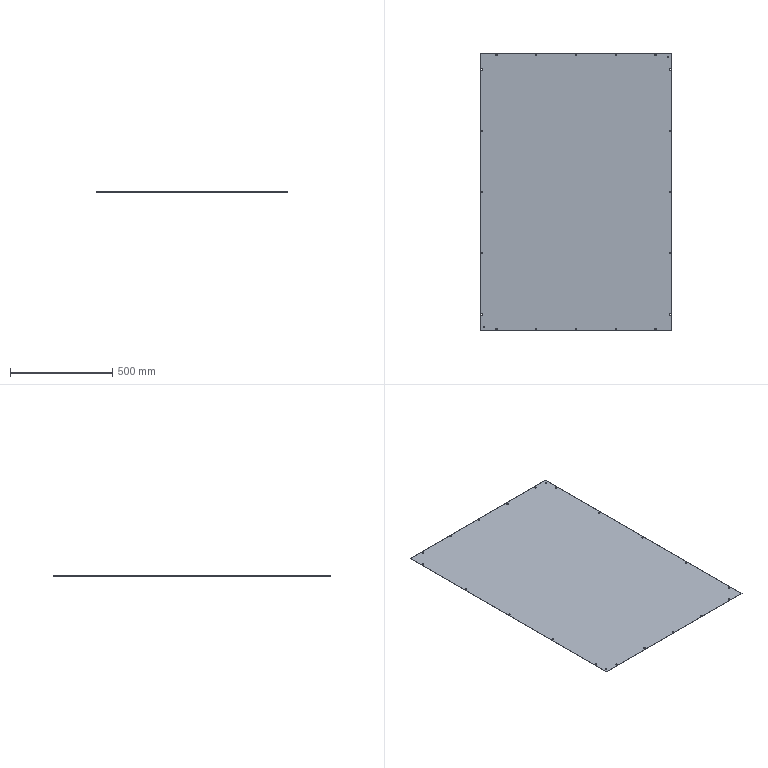Part | SolidWorks | features Cut 2, Extrusion 1 | 1 solid | 100 faces | box 940 x 1360 x 1 mm | volume 1277171 mm3 | cylinder 54 | plane 46 | commonest cylinder face diameters 7 x50 5 x4